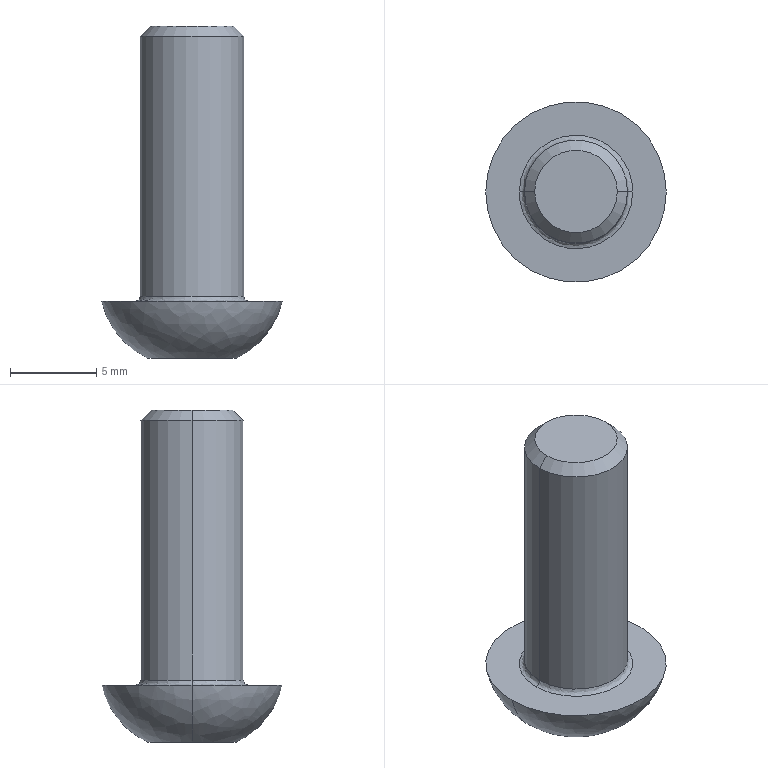Part | SolidWorks | features BaseBody 1 | 1 solid | 25 faces | box 10.5 x 10.5 x 19.3 mm | volume 617.652 mm3 | plane 15 | spline 4 | cone 4 | cylinder 2 | commonest cylinder face diameters 6 x2
STEP:
#1=CARTESIAN_POINT('',(3.,0.,3.6));
#2=VERTEX_POINT('',#1);
#3=CARTESIAN_POINT('',(-3.,0.,3.6));
#4=VERTEX_POINT('',#3);
#5=CARTESIAN_POINT('',(0.,0.,3.6));
#6=DIRECTION('',(0.,0.,1.));
#7=DIRECTION('',(-1.,0.,0.));
#8=AXIS2_PLACEMENT_3D('',#5,#6,#7);
#9=CIRCLE('',#8,3.);
#10=EDGE_CURVE('',#2,#4,#9,.T.);
#11=ORIENTED_EDGE('',*,*,#10,.F.);
#12=CARTESIAN_POINT('',(3.3,0.,3.3));
#13=VERTEX_POINT('',#12);
#14=CARTESIAN_POINT('',(3.3,0.,3.6));
#15=DIRECTION('',(0.,-1.,0.));
#16=DIRECTION('',(1.,0.,0.));
#17=AXIS2_PLACEMENT_3D('',#14,#15,#16);
#18=CIRCLE('',#17,0.3);
#19=EDGE_CURVE('',#2,#13,#18,.T.);
#20=ORIENTED_EDGE('',*,*,#19,.T.);
#21=CARTESIAN_POINT('',(-3.3,0.,3.3));
#22=VERTEX_POINT('',#21);
#23=CARTESIAN_POINT('',(-3.3,0.,3.3));
#24=CARTESIAN_POINT('',(-3.3,0.2099,3.3));
#25=CARTESIAN_POINT('',(-3.271,0.5192,3.3));
#26=CARTESIAN_POINT('',(-3.187,0.8702,3.3));
#27=CARTESIAN_POINT('',(-3.132,1.043,3.3));
#28=CARTESIAN_POINT('',(-3.101,1.129,3.3));
#29=CARTESIAN_POINT('',(-3.087,1.166,3.3));
#30=CARTESIAN_POINT('',(-3.078,1.19,3.3));
#31=CARTESIAN_POINT('',(-3.074,1.201,3.3));
#32=CARTESIAN_POINT('',(-2.9,1.639,3.3));
#33=CARTESIAN_POINT('',(-2.656,2.011,3.3));
#34=CARTESIAN_POINT('',(-2.172,2.495,3.3));
#35=CARTESIAN_POINT('',(-1.911,2.707,3.3));
#36=CARTESIAN_POINT('',(-1.574,2.905,3.3));
#37=CARTESIAN_POINT('',(-1.397,2.991,3.3));
#38=CARTESIAN_POINT('',(-1.32,3.025,3.3));
#39=CARTESIAN_POINT('',(-1.267,3.047,3.3));
#40=CARTESIAN_POINT('',(-1.239,3.059,3.3));
#41=CARTESIAN_POINT('',(-0.8242,3.223,3.3));
#42=CARTESIAN_POINT('',(-0.42,3.3,3.3));
#43=CARTESIAN_POINT('',(0.21,3.3,3.3));
#44=CARTESIAN_POINT('',(0.5193,3.271,3.3));
#45=CARTESIAN_POINT('',(0.8703,3.187,3.3));
#46=CARTESIAN_POINT('',(1.043,3.132,3.3));
#47=CARTESIAN_POINT('',(1.129,3.101,3.3));
#48=CARTESIAN_POINT('',(1.166,3.087,3.3));
#49=CARTESIAN_POINT('',(1.19,3.078,3.3));
#50=CARTESIAN_POINT('',(1.201,3.074,3.3));
#51=CARTESIAN_POINT('',(1.639,2.9,3.3));
#52=CARTESIAN_POINT('',(2.011,2.656,3.3));
#53=CARTESIAN_POINT('',(2.495,2.172,3.3));
#54=CARTESIAN_POINT('',(2.707,1.911,3.3));
#55=CARTESIAN_POINT('',(2.905,1.574,3.3));
#56=CARTESIAN_POINT('',(2.991,1.397,3.3));
#57=CARTESIAN_POINT('',(3.025,1.32,3.3));
#58=CARTESIAN_POINT('',(3.047,1.267,3.3));
#59=CARTESIAN_POINT('',(3.059,1.239,3.3));
#60=CARTESIAN_POINT('',(3.223,0.8244,3.3));
#61=CARTESIAN_POINT('',(3.3,0.4195,3.3));
#62=CARTESIAN_POINT('',(3.3,0.,3.3));
#63=B_SPLINE_CURVE_WITH_KNOTS('',3,(#23,#24,#25,#26,#27,#28,#29,#30,#31,#32,#33,#34,#35,#36,#37,#38,#39,#40,#41,#42,#43,#44,#45,#46,#47,#48,#49,#50,#51,#52,#53,#54,#55,#56,#57,#58,#59,#60,#61,#62),.UNSPECIFIED.,.F.,.F.,(4,1,1,1,1,2,2,2,1,1,1,2,2,2,1,1,1,1,2,2,2,1,1,1,2,2,4),(0.,0.0625,0.09375,0.1094,0.1172,0.1211,0.125,0.25,0.3125,0.3437,0.3594,0.3672,0.375,0.5,0.5625,0.5937,0.6094,0.6172,0.6211,0.625,0.75,0.8125,0.8437,0.8594,0.8672,0.875,1.),.UNSPECIFIED.);
#64=EDGE_CURVE('',#22,#13,#63,.T.);
#65=ORIENTED_EDGE('',*,*,#64,.F.);
#66=CARTESIAN_POINT('',(-3.3,0.,3.6));
#67=DIRECTION('',(0.,1.,0.));
#68=DIRECTION('',(-1.,0.,0.));
#69=AXIS2_PLACEMENT_3D('',#66,#67,#68);
#70=CIRCLE('',#69,0.3);
#71=EDGE_CURVE('',#4,#22,#70,.T.);
#72=ORIENTED_EDGE('',*,*,#71,.F.);
#73=EDGE_LOOP('',(#11,#20,#65,#72));
#74=FACE_OUTER_BOUND('',#73,.T.);
#75=CARTESIAN_POINT('',(-3.,0.,3.6));
#76=CARTESIAN_POINT('',(-3.,6.,3.6));
#77=CARTESIAN_POINT('',(3.,6.,3.6));
#78=CARTESIAN_POINT('',(3.,0.,3.6));
#79=CARTESIAN_POINT('',(-3.,0.,3.424));
#80=CARTESIAN_POINT('',(-3.,6.,3.424));
#81=CARTESIAN_POINT('',(3.,6.,3.424));
#82=CARTESIAN_POINT('',(3.,0.,3.424));
#83=CARTESIAN_POINT('',(-3.124,0.,3.3));
#84=CARTESIAN_POINT('',(-3.124,6.249,3.3));
#85=CARTESIAN_POINT('',(3.124,6.249,3.3));
#86=CARTESIAN_POINT('',(3.124,0.,3.3));
#87=CARTESIAN_POINT('',(-3.3,0.,3.3));
#88=CARTESIAN_POINT('',(-3.3,6.6,3.3));
#89=CARTESIAN_POINT('',(3.3,6.6,3.3));
#90=CARTESIAN_POINT('',(3.3,0.,3.3));
#91=(BOUNDED_SURFACE()B_SPLINE_SURFACE(3,3,((#75,#76,#77,#78),(#79,#80,#81,#82),(#83,#84,#85,#86),(#87,#88,#89,#90)),.UNSPECIFIED.,.F.,.F.,.F.)B_SPLINE_SURFACE_WITH_KNOTS((4,4),(4,4),(0.,1.),(0.,1.),.UNSPECIFIED.)GEOMETRIC_REPRESENTATION_ITEM()RATIONAL_B_SPLINE_SURFACE(((1.,0.3333,0.3333,1.),(0.8047,0.2682,0.2682,0.8047),(0.8047,0.2682,0.2682,0.8047),(1.,0.3333,0.3333,1.)))REPRESENTATION_ITEM('')SURFACE());
#92=ADVANCED_FACE('',(#74),#91,.F.);
#93=CARTESIAN_POINT('',(5.25,0.,3.3));
#94=VERTEX_POINT('',#93);
#95=CARTESIAN_POINT('',(-5.25,0.,3.3));
#96=VERTEX_POINT('',#95);
#97=CARTESIAN_POINT('',(0.,0.,3.3));
#98=DIRECTION('',(0.,0.,-1.));
#99=DIRECTION('',(1.,0.,0.));
#100=AXIS2_PLACEMENT_3D('',#97,#98,#99);
#101=CIRCLE('',#100,5.25);
#102=EDGE_CURVE('',#94,#96,#101,.T.);
#103=ORIENTED_EDGE('',*,*,#102,.T.);
#104=CARTESIAN_POINT('',(-2.6,0.,0.));
#105=VERTEX_POINT('',#104);
#106=CARTESIAN_POINT('',(-0.5657,0.,4.348));
#107=DIRECTION('',(0.,-1.,0.));
#108=DIRECTION('',(-1.,0.,0.));
#109=AXIS2_PLACEMENT_3D('',#106,#107,#108);
#110=CIRCLE('',#109,4.8);
#111=EDGE_CURVE('',#96,#105,#110,.T.);
#112=ORIENTED_EDGE('',*,*,#111,.T.);
#113=CARTESIAN_POINT('',(2.6,0.,0.));
#114=VERTEX_POINT('',#113);
#115=CARTESIAN_POINT('',(0.,0.,0.));
#116=DIRECTION('',(0.,0.,1.));
#117=DIRECTION('',(1.,0.,0.));
#118=AXIS2_PLACEMENT_3D('',#115,#116,#117);
#119=CIRCLE('',#118,2.6);
#120=EDGE_CURVE('',#105,#114,#119,.T.);
#121=ORIENTED_EDGE('',*,*,#120,.T.);
#122=CARTESIAN_POINT('',(0.5657,0.,4.348));
#123=DIRECTION('',(0.,1.,0.));
#124=DIRECTION('',(1.,0.,0.));
#125=AXIS2_PLACEMENT_3D('',#122,#123,#124);
#126=CIRCLE('',#125,4.8);
#127=EDGE_CURVE('',#94,#114,#126,.T.);
#128=ORIENTED_EDGE('',*,*,#127,.F.);
#129=EDGE_LOOP('',(#103,#112,#121,#128));
#130=FACE_OUTER_BOUND('',#129,.T.);
#131=CARTESIAN_POINT('',(-5.25,0.,3.3));
#132=CARTESIAN_POINT('',(-5.25,-10.5,3.3));
#133=CARTESIAN_POINT('',(5.25,-10.5,3.3));
#134=CARTESIAN_POINT('',(5.25,0.,3.3));
#135=CARTESIAN_POINT('',(-4.92,0.,1.822));
#136=CARTESIAN_POINT('',(-4.92,-9.839,1.822));
#137=CARTESIAN_POINT('',(4.92,-9.839,1.822));
#138=CARTESIAN_POINT('',(4.92,0.,1.822));
#139=CARTESIAN_POINT('',(-3.971,0.,0.6417));
#140=CARTESIAN_POINT('',(-3.971,-7.943,0.6417));
#141=CARTESIAN_POINT('',(3.971,-7.943,0.6417));
#142=CARTESIAN_POINT('',(3.971,0.,0.6417));
#143=CARTESIAN_POINT('',(-2.6,0.,0.));
#144=CARTESIAN_POINT('',(-2.6,-5.2,0.));
#145=CARTESIAN_POINT('',(2.6,-5.2,0.));
#146=CARTESIAN_POINT('',(2.6,0.,0.));
#147=(BOUNDED_SURFACE()B_SPLINE_SURFACE(3,3,((#131,#132,#133,#134),(#135,#136,#137,#138),(#139,#140,#141,#142),(#143,#144,#145,#146)),.UNSPECIFIED.,.F.,.F.,.F.)B_SPLINE_SURFACE_WITH_KNOTS((4,4),(4,4),(0.,1.),(0.,1.),.UNSPECIFIED.)GEOMETRIC_REPRESENTATION_ITEM()RATIONAL_B_SPLINE_SURFACE(((1.,0.3333,0.3333,1.),(0.9317,0.3106,0.3106,0.9317),(0.9317,0.3106,0.3106,0.9317),(1.,0.3333,0.3333,1.)))REPRESENTATION_ITEM('')SURFACE());
#148=ADVANCED_FACE('',(#130),#147,.T.);
#149=CARTESIAN_POINT('',(-3.,0.,18.7));
#150=VERTEX_POINT('',#149);
#151=CARTESIAN_POINT('',(3.,0.,18.7));
#152=VERTEX_POINT('',#151);
#153=CARTESIAN_POINT('',(0.,0.,18.7));
#154=DIRECTION('',(0.,0.,-1.));
#155=DIRECTION('',(-1.,0.,0.));
#156=AXIS2_PLACEMENT_3D('',#153,#154,#155);
#157=CIRCLE('',#156,3.);
#158=EDGE_CURVE('',#150,#152,#157,.T.);
#159=ORIENTED_EDGE('',*,*,#158,.T.);
#160=CARTESIAN_POINT('',(3.,0.,19.3));
#161=DIRECTION('',(0.,0.,-1.));
#162=VECTOR('',#161,1000.);
#163=LINE('',#160,#162);
#164=EDGE_CURVE('',#152,#2,#163,.T.);
#165=ORIENTED_EDGE('',*,*,#164,.T.);
#166=ORIENTED_EDGE('',*,*,#10,.T.);
#167=CARTESIAN_POINT('',(-3.,0.,19.3));
#168=DIRECTION('',(0.,0.,-1.));
#169=VECTOR('',#168,1000.);
#170=LINE('',#167,#169);
#171=EDGE_CURVE('',#150,#4,#170,.T.);
#172=ORIENTED_EDGE('',*,*,#171,.F.);
#173=EDGE_LOOP('',(#159,#165,#166,#172));
#174=FACE_OUTER_BOUND('',#173,.T.);
#175=CARTESIAN_POINT('',(0.,0.,19.3));
#176=DIRECTION('',(0.,0.,-1.));
#177=DIRECTION('',(-1.,0.,0.));
#178=AXIS2_PLACEMENT_3D('',#175,#176,#177);
#179=CYLINDRICAL_SURFACE('',#178,3.);
#180=ADVANCED_FACE('',(#174),#179,.T.);
#181=CARTESIAN_POINT('',(-2.4,0.,19.3));
#182=VERTEX_POINT('',#181);
#183=CARTESIAN_POINT('',(2.4,0.,19.3));
#184=VERTEX_POINT('',#183);
#185=CARTESIAN_POINT('',(0.,0.,19.3));
#186=DIRECTION('',(0.,0.,-1.));
#187=DIRECTION('',(-1.,0.,0.));
#188=AXIS2_PLACEMENT_3D('',#185,#186,#187);
#189=CIRCLE('',#188,2.4);
#190=EDGE_CURVE('',#182,#184,#189,.T.);
#191=ORIENTED_EDGE('',*,*,#190,.T.);
#192=CARTESIAN_POINT('',(3.,0.,18.7));
#193=DIRECTION('',(0.7071,0.,-0.7071));
#194=VECTOR('',#193,1000.);
#195=LINE('',#192,#194);
#196=EDGE_CURVE('',#184,#152,#195,.T.);
#197=ORIENTED_EDGE('',*,*,#196,.T.);
#198=ORIENTED_EDGE('',*,*,#158,.F.);
#199=CARTESIAN_POINT('',(-3.,0.,18.7));
#200=DIRECTION('',(-0.7071,0.,-0.7071));
#201=VECTOR('',#200,1000.);
#202=LINE('',#199,#201);
#203=EDGE_CURVE('',#182,#150,#202,.T.);
#204=ORIENTED_EDGE('',*,*,#203,.F.);
#205=EDGE_LOOP('',(#191,#197,#198,#204));
#206=FACE_OUTER_BOUND('',#205,.T.);
#207=CARTESIAN_POINT('',(0.,0.,18.7));
#208=DIRECTION('',(0.,0.,-1.));
#209=DIRECTION('',(-1.,0.,0.));
#210=AXIS2_PLACEMENT_3D('',#207,#208,#209);
#211=CONICAL_SURFACE('',#210,3.,0.7854);
#212=ADVANCED_FACE('',(#206),#211,.T.);
#213=CARTESIAN_POINT('',(0.,0.,3.235));
#214=VERTEX_POINT('',#213);
#215=CARTESIAN_POINT('',(-2.,0.,2.08));
#216=VERTEX_POINT('',#215);
#217=CARTESIAN_POINT('',(-2.,0.,2.08));
#218=DIRECTION('',(-0.866,0.,-0.5));
#219=VECTOR('',#218,1000.);
#220=LINE('',#217,#219);
#221=EDGE_CURVE('',#214,#216,#220,.T.);
#222=ORIENTED_EDGE('',*,*,#221,.F.);
#223=CARTESIAN_POINT('',(2.,0.,2.08));
#224=VERTEX_POINT('',#223);
#225=CARTESIAN_POINT('',(2.,0.,2.08));
#226=DIRECTION('',(0.866,0.,-0.5));
#227=VECTOR('',#226,1000.);
#228=LINE('',#225,#227);
#229=EDGE_CURVE('',#214,#224,#228,.T.);
#230=ORIENTED_EDGE('',*,*,#229,.T.);
#231=CARTESIAN_POINT('',(1.,-1.732,2.08));
#232=VERTEX_POINT('',#231);
#233=CARTESIAN_POINT('',(0.,0.,2.08));
#234=DIRECTION('',(0.,0.,1.));
#235=DIRECTION('',(-1.,0.,0.));
#236=AXIS2_PLACEMENT_3D('',#233,#234,#235);
#237=CIRCLE('',#236,2.);
#238=EDGE_CURVE('',#232,#224,#237,.T.);
#239=ORIENTED_EDGE('',*,*,#238,.F.);
#240=CARTESIAN_POINT('',(-1.,-1.732,2.08));
#241=VERTEX_POINT('',#240);
#242=CARTESIAN_POINT('',(0.,0.,2.08));
#243=DIRECTION('',(0.,0.,1.));
#244=DIRECTION('',(-1.,0.,0.));
#245=AXIS2_PLACEMENT_3D('',#242,#243,#244);
#246=CIRCLE('',#245,2.);
#247=EDGE_CURVE('',#241,#232,#246,.T.);
#248=ORIENTED_EDGE('',*,*,#247,.F.);
#249=CARTESIAN_POINT('',(0.,0.,2.08));
#250=DIRECTION('',(0.,0.,1.));
#251=DIRECTION('',(-1.,0.,0.));
#252=AXIS2_PLACEMENT_3D('',#249,#250,#251);
#253=CIRCLE('',#252,2.);
#254=EDGE_CURVE('',#216,#241,#253,.T.);
#255=ORIENTED_EDGE('',*,*,#254,.F.);
#256=EDGE_LOOP('',(#222,#230,#239,#248,#255));
#257=FACE_OUTER_BOUND('',#256,.T.);
#258=CARTESIAN_POINT('',(0.,0.,2.08));
#259=DIRECTION('',(0.,0.,-1.));
#260=DIRECTION('',(-1.,0.,0.));
#261=AXIS2_PLACEMENT_3D('',#258,#259,#260);
#262=CONICAL_SURFACE('',#261,2.,1.047);
#263=ADVANCED_FACE('',(#257),#262,.F.);
#264=ORIENTED_EDGE('',*,*,#164,.F.);
#265=CARTESIAN_POINT('',(0.,0.,18.7));
#266=DIRECTION('',(0.,0.,-1.));
#267=DIRECTION('',(-1.,0.,0.));
#268=AXIS2_PLACEMENT_3D('',#265,#266,#267);
#269=CIRCLE('',#268,3.);
#270=EDGE_CURVE('',#152,#150,#269,.T.);
#271=ORIENTED_EDGE('',*,*,#270,.T.);
#272=ORIENTED_EDGE('',*,*,#171,.T.);
#273=CARTESIAN_POINT('',(0.,0.,3.6));
#274=DIRECTION('',(0.,0.,1.));
#275=DIRECTION('',(-1.,0.,0.));
#276=AXIS2_PLACEMENT_3D('',#273,#274,#275);
#277=CIRCLE('',#276,3.);
#278=EDGE_CURVE('',#4,#2,#277,.T.);
#279=ORIENTED_EDGE('',*,*,#278,.T.);
#280=EDGE_LOOP('',(#264,#271,#272,#279));
#281=FACE_OUTER_BOUND('',#280,.T.);
#282=CARTESIAN_POINT('',(0.,0.,19.3));
#283=DIRECTION('',(0.,0.,-1.));
#284=DIRECTION('',(-1.,0.,0.));
#285=AXIS2_PLACEMENT_3D('',#282,#283,#284);
#286=CYLINDRICAL_SURFACE('',#285,3.);
#287=ADVANCED_FACE('',(#281),#286,.T.);
#288=ORIENTED_EDGE('',*,*,#19,.F.);
#289=ORIENTED_EDGE('',*,*,#278,.F.);
#290=ORIENTED_EDGE('',*,*,#71,.T.);
#291=CARTESIAN_POINT('',(3.3,0.,3.3));
#292=CARTESIAN_POINT('',(3.3,-0.2099,3.3));
#293=CARTESIAN_POINT('',(3.271,-0.5192,3.3));
#294=CARTESIAN_POINT('',(3.187,-0.8702,3.3));
#295=CARTESIAN_POINT('',(3.132,-1.043,3.3));
#296=CARTESIAN_POINT('',(3.101,-1.129,3.3));
#297=CARTESIAN_POINT('',(3.087,-1.166,3.3));
#298=CARTESIAN_POINT('',(3.078,-1.19,3.3));
#299=CARTESIAN_POINT('',(3.074,-1.201,3.3));
#300=CARTESIAN_POINT('',(2.9,-1.639,3.3));
#301=CARTESIAN_POINT('',(2.656,-2.011,3.3));
#302=CARTESIAN_POINT('',(2.172,-2.495,3.3));
#303=CARTESIAN_POINT('',(1.911,-2.707,3.3));
#304=CARTESIAN_POINT('',(1.574,-2.905,3.3));
#305=CARTESIAN_POINT('',(1.397,-2.991,3.3));
#306=CARTESIAN_POINT('',(1.32,-3.025,3.3));
#307=CARTESIAN_POINT('',(1.267,-3.047,3.3));
#308=CARTESIAN_POINT('',(1.239,-3.059,3.3));
#309=CARTESIAN_POINT('',(0.8242,-3.223,3.3));
#310=CARTESIAN_POINT('',(0.42,-3.3,3.3));
#311=CARTESIAN_POINT('',(-0.21,-3.3,3.3));
#312=CARTESIAN_POINT('',(-0.5193,-3.271,3.3));
#313=CARTESIAN_POINT('',(-0.8703,-3.187,3.3));
#314=CARTESIAN_POINT('',(-1.043,-3.132,3.3));
#315=CARTESIAN_POINT('',(-1.129,-3.101,3.3));
#316=CARTESIAN_POINT('',(-1.166,-3.087,3.3));
#317=CARTESIAN_POINT('',(-1.19,-3.078,3.3));
#318=CARTESIAN_POINT('',(-1.201,-3.074,3.3));
#319=CARTESIAN_POINT('',(-1.639,-2.9,3.3));
#320=CARTESIAN_POINT('',(-2.011,-2.656,3.3));
#321=CARTESIAN_POINT('',(-2.495,-2.172,3.3));
#322=CARTESIAN_POINT('',(-2.707,-1.911,3.3));
#323=CARTESIAN_POINT('',(-2.905,-1.574,3.3));
#324=CARTESIAN_POINT('',(-2.991,-1.397,3.3));
#325=CARTESIAN_POINT('',(-3.025,-1.32,3.3));
#326=CARTESIAN_POINT('',(-3.047,-1.267,3.3));
#327=CARTESIAN_POINT('',(-3.059,-1.239,3.3));
#328=CARTESIAN_POINT('',(-3.223,-0.8244,3.3));
#329=CARTESIAN_POINT('',(-3.3,-0.4195,3.3));
#330=CARTESIAN_POINT('',(-3.3,0.,3.3));
#331=B_SPLINE_CURVE_WITH_KNOTS('',3,(#291,#292,#293,#294,#295,#296,#297,#298,#299,#300,#301,#302,#303,#304,#305,#306,#307,#308,#309,#310,#311,#312,#313,#314,#315,#316,#317,#318,#319,#320,#321,#322,#323,#324,#325,#326,#327,#328,#329,#330),.UNSPECIFIED.,.F.,.F.,(4,1,1,1,1,2,2,2,1,1,1,2,2,2,1,1,1,1,2,2,2,1,1,1,2,2,4),(0.,0.0625,0.09375,0.1094,0.1172,0.1211,0.125,0.25,0.3125,0.3437,0.3594,0.3672,0.375,0.5,0.5625,0.5937,0.6094,0.6172,0.6211,0.625,0.75,0.8125,0.8438,0.8594,0.8672,0.875,1.),.UNSPECIFIED.);
#332=EDGE_CURVE('',#13,#22,#331,.T.);
#333=ORIENTED_EDGE('',*,*,#332,.F.);
#334=EDGE_LOOP('',(#288,#289,#290,#333));
#335=FACE_OUTER_BOUND('',#334,.T.);
#336=CARTESIAN_POINT('',(3.,0.,3.6));
#337=CARTESIAN_POINT('',(3.,-6.,3.6));
#338=CARTESIAN_POINT('',(-3.,-6.,3.6));
#339=CARTESIAN_POINT('',(-3.,0.,3.6));
#340=CARTESIAN_POINT('',(3.,0.,3.424));
#341=CARTESIAN_POINT('',(3.,-6.,3.424));
#342=CARTESIAN_POINT('',(-3.,-6.,3.424));
#343=CARTESIAN_POINT('',(-3.,0.,3.424));
#344=CARTESIAN_POINT('',(3.124,0.,3.3));
#345=CARTESIAN_POINT('',(3.124,-6.249,3.3));
#346=CARTESIAN_POINT('',(-3.124,-6.249,3.3));
#347=CARTESIAN_POINT('',(-3.124,0.,3.3));
#348=CARTESIAN_POINT('',(3.3,0.,3.3));
#349=CARTESIAN_POINT('',(3.3,-6.6,3.3));
#350=CARTESIAN_POINT('',(-3.3,-6.6,3.3));
#351=CARTESIAN_POINT('',(-3.3,0.,3.3));
#352=(BOUNDED_SURFACE()B_SPLINE_SURFACE(3,3,((#336,#337,#338,#339),(#340,#341,#342,#343),(#344,#345,#346,#347),(#348,#349,#350,#351)),.UNSPECIFIED.,.F.,.F.,.F.)B_SPLINE_SURFACE_WITH_KNOTS((4,4),(4,4),(0.,1.),(0.,1.),.UNSPECIFIED.)GEOMETRIC_REPRESENTATION_ITEM()RATIONAL_B_SPLINE_SURFACE(((1.,0.3333,0.3333,1.),(0.8047,0.2682,0.2682,0.8047),(0.8047,0.2682,0.2682,0.8047),(1.,0.3333,0.3333,1.)))REPRESENTATION_ITEM('')SURFACE());
#353=ADVANCED_FACE('',(#335),#352,.F.);
#354=ORIENTED_EDGE('',*,*,#196,.F.);
#355=CARTESIAN_POINT('',(0.,0.,19.3));
#356=DIRECTION('',(0.,0.,-1.));
#357=DIRECTION('',(-1.,0.,0.));
#358=AXIS2_PLACEMENT_3D('',#355,#356,#357);
#359=CIRCLE('',#358,2.4);
#360=EDGE_CURVE('',#184,#182,#359,.T.);
#361=ORIENTED_EDGE('',*,*,#360,.T.);
#362=ORIENTED_EDGE('',*,*,#203,.T.);
#363=ORIENTED_EDGE('',*,*,#270,.F.);
#364=EDGE_LOOP('',(#354,#361,#362,#363));
#365=FACE_OUTER_BOUND('',#364,.T.);
#366=CARTESIAN_POINT('',(0.,0.,18.7));
#367=DIRECTION('',(0.,0.,-1.));
#368=DIRECTION('',(-1.,0.,0.));
#369=AXIS2_PLACEMENT_3D('',#366,#367,#368);
#370=CONICAL_SURFACE('',#369,3.,0.7854);
#371=ADVANCED_FACE('',(#365),#370,.T.);
#372=ORIENTED_EDGE('',*,*,#102,.F.);
#373=CARTESIAN_POINT('',(0.,0.,3.3));
#374=DIRECTION('',(0.,0.,-1.));
#375=DIRECTION('',(1.,0.,0.));
#376=AXIS2_PLACEMENT_3D('',#373,#374,#375);
#377=CIRCLE('',#376,5.25);
#378=EDGE_CURVE('',#96,#94,#377,.T.);
#379=ORIENTED_EDGE('',*,*,#378,.F.);
#380=EDGE_LOOP('',(#372,#379));
#381=FACE_OUTER_BOUND('',#380,.T.);
#382=ORIENTED_EDGE('',*,*,#332,.T.);
#383=ORIENTED_EDGE('',*,*,#64,.T.);
#384=EDGE_LOOP('',(#382,#383));
#385=FACE_BOUND('',#384,.T.);
#386=CARTESIAN_POINT('',(-5.25,0.,3.3));
#387=DIRECTION('',(0.,0.,-1.));
#388=DIRECTION('',(-1.,0.,0.));
#389=AXIS2_PLACEMENT_3D('',#386,#387,#388);
#390=PLANE('',#389);
#391=ADVANCED_FACE('',(#381,#385),#390,.F.);
#392=ORIENTED_EDGE('',*,*,#190,.F.);
#393=ORIENTED_EDGE('',*,*,#360,.F.);
#394=EDGE_LOOP('',(#392,#393));
#395=FACE_OUTER_BOUND('',#394,.T.);
#396=CARTESIAN_POINT('',(0.,0.,19.3));
#397=DIRECTION('',(0.,0.,1.));
#398=DIRECTION('',(1.,0.,0.));
#399=AXIS2_PLACEMENT_3D('',#396,#397,#398);
#400=PLANE('',#399);
#401=ADVANCED_FACE('',(#395),#400,.T.);
#402=ORIENTED_EDGE('',*,*,#111,.F.);
#403=ORIENTED_EDGE('',*,*,#378,.T.);
#404=ORIENTED_EDGE('',*,*,#127,.T.);
#405=CARTESIAN_POINT('',(0.,0.,0.));
#406=DIRECTION('',(0.,0.,1.));
#407=DIRECTION('',(1.,0.,0.));
#408=AXIS2_PLACEMENT_3D('',#405,#406,#407);
#409=CIRCLE('',#408,2.6);
#410=EDGE_CURVE('',#114,#105,#409,.T.);
#411=ORIENTED_EDGE('',*,*,#410,.T.);
#412=EDGE_LOOP('',(#402,#403,#404,#411));
#413=FACE_OUTER_BOUND('',#412,.T.);
#414=CARTESIAN_POINT('',(5.25,0.,3.3));
#415=CARTESIAN_POINT('',(5.25,10.5,3.3));
#416=CARTESIAN_POINT('',(-5.25,10.5,3.3));
#417=CARTESIAN_POINT('',(-5.25,0.,3.3));
#418=CARTESIAN_POINT('',(4.92,0.,1.822));
#419=CARTESIAN_POINT('',(4.92,9.839,1.822));
#420=CARTESIAN_POINT('',(-4.92,9.839,1.822));
#421=CARTESIAN_POINT('',(-4.92,0.,1.822));
#422=CARTESIAN_POINT('',(3.971,0.,0.6417));
#423=CARTESIAN_POINT('',(3.971,7.943,0.6417));
#424=CARTESIAN_POINT('',(-3.971,7.943,0.6417));
#425=CARTESIAN_POINT('',(-3.971,0.,0.6417));
#426=CARTESIAN_POINT('',(2.6,0.,0.));
#427=CARTESIAN_POINT('',(2.6,5.2,0.));
#428=CARTESIAN_POINT('',(-2.6,5.2,0.));
#429=CARTESIAN_POINT('',(-2.6,0.,0.));
#430=(BOUNDED_SURFACE()B_SPLINE_SURFACE(3,3,((#414,#415,#416,#417),(#418,#419,#420,#421),(#422,#423,#424,#425),(#426,#427,#428,#429)),.UNSPECIFIED.,.F.,.F.,.F.)B_SPLINE_SURFACE_WITH_KNOTS((4,4),(4,4),(0.,1.),(0.,1.),.UNSPECIFIED.)GEOMETRIC_REPRESENTATION_ITEM()RATIONAL_B_SPLINE_SURFACE(((1.,0.3333,0.3333,1.),(0.9317,0.3106,0.3106,0.9317),(0.9317,0.3106,0.3106,0.9317),(1.,0.3333,0.3333,1.)))REPRESENTATION_ITEM('')SURFACE());
#431=ADVANCED_FACE('',(#413),#430,.T.);
#432=ORIENTED_EDGE('',*,*,#410,.F.);
#433=ORIENTED_EDGE('',*,*,#120,.F.);
#434=EDGE_LOOP('',(#432,#433));
#435=FACE_OUTER_BOUND('',#434,.T.);
#436=CARTESIAN_POINT('',(-2.,-1.155,0.));
#437=VERTEX_POINT('',#436);
#438=CARTESIAN_POINT('',(-2.,1.155,0.));
#439=VERTEX_POINT('',#438);
#440=CARTESIAN_POINT('',(-2.,0.,0.));
#441=DIRECTION('',(0.,1.,0.));
#442=VECTOR('',#441,1000.);
#443=LINE('',#440,#442);
#444=EDGE_CURVE('',#437,#439,#443,.T.);
#445=ORIENTED_EDGE('',*,*,#444,.F.);
#446=CARTESIAN_POINT('',(0.,-2.309,0.));
#447=VERTEX_POINT('',#446);
#448=CARTESIAN_POINT('',(0.,-2.309,0.));
#449=DIRECTION('',(-0.866,0.5,0.));
#450=VECTOR('',#449,1000.);
#451=LINE('',#448,#450);
#452=EDGE_CURVE('',#447,#437,#451,.T.);
#453=ORIENTED_EDGE('',*,*,#452,.F.);
#454=CARTESIAN_POINT('',(2.,-1.155,0.));
#455=VERTEX_POINT('',#454);
#456=CARTESIAN_POINT('',(2.,-1.155,0.));
#457=DIRECTION('',(-0.866,-0.5,0.));
#458=VECTOR('',#457,1000.);
#459=LINE('',#456,#458);
#460=EDGE_CURVE('',#455,#447,#459,.T.);
#461=ORIENTED_EDGE('',*,*,#460,.F.);
#462=CARTESIAN_POINT('',(2.,1.155,0.));
#463=VERTEX_POINT('',#462);
#464=CARTESIAN_POINT('',(2.,0.,0.));
#465=DIRECTION('',(0.,-1.,0.));
#466=VECTOR('',#465,1000.);
#467=LINE('',#464,#466);
#468=EDGE_CURVE('',#463,#455,#467,.T.);
#469=ORIENTED_EDGE('',*,*,#468,.F.);
#470=CARTESIAN_POINT('',(0.,2.309,0.));
#471=VERTEX_POINT('',#470);
#472=CARTESIAN_POINT('',(0.,2.309,0.));
#473=DIRECTION('',(0.866,-0.5,0.));
#474=VECTOR('',#473,1000.);
#475=LINE('',#472,#474);
#476=EDGE_CURVE('',#471,#463,#475,.T.);
#477=ORIENTED_EDGE('',*,*,#476,.F.);
#478=CARTESIAN_POINT('',(-2.,1.155,0.));
#479=DIRECTION('',(0.866,0.5,0.));
#480=VECTOR('',#479,1000.);
#481=LINE('',#478,#480);
#482=EDGE_CURVE('',#439,#471,#481,.T.);
#483=ORIENTED_EDGE('',*,*,#482,.F.);
#484=EDGE_LOOP('',(#445,#453,#461,#469,#477,#483));
#485=FACE_BOUND('',#484,.T.);
#486=CARTESIAN_POINT('',(-2.6,0.,0.));
#487=DIRECTION('',(0.,0.,1.));
#488=DIRECTION('',(1.,0.,0.));
#489=AXIS2_PLACEMENT_3D('',#486,#487,#488);
#490=PLANE('',#489);
#491=ADVANCED_FACE('',(#435,#485),#490,.F.);
#492=CARTESIAN_POINT('',(0.,2.309,2.08));
#493=VERTEX_POINT('',#492);
#494=CARTESIAN_POINT('',(0.,2.309,2.08));
#495=DIRECTION('',(0.,0.,-1.));
#496=VECTOR('',#495,1000.);
#497=LINE('',#494,#496);
#498=EDGE_CURVE('',#493,#471,#497,.T.);
#499=ORIENTED_EDGE('',*,*,#498,.F.);
#500=CARTESIAN_POINT('',(-1.,1.732,2.08));
#501=VERTEX_POINT('',#500);
#502=CARTESIAN_POINT('',(-1.,1.732,2.08));
#503=DIRECTION('',(0.866,0.5,0.));
#504=VECTOR('',#503,1000.);
#505=LINE('',#502,#504);
#506=EDGE_CURVE('',#501,#493,#505,.T.);
#507=ORIENTED_EDGE('',*,*,#506,.F.);
#508=CARTESIAN_POINT('',(-2.,1.155,2.08));
#509=VERTEX_POINT('',#508);
#510=CARTESIAN_POINT('',(-2.,1.155,2.08));
#511=DIRECTION('',(0.866,0.5,0.));
#512=VECTOR('',#511,1000.);
#513=LINE('',#510,#512);
#514=EDGE_CURVE('',#509,#501,#513,.T.);
#515=ORIENTED_EDGE('',*,*,#514,.F.);
#516=CARTESIAN_POINT('',(-2.,1.155,2.08));
#517=DIRECTION('',(0.,0.,1.));
#518=VECTOR('',#517,1000.);
#519=LINE('',#516,#518);
#520=EDGE_CURVE('',#439,#509,#519,.T.);
#521=ORIENTED_EDGE('',*,*,#520,.F.);
#522=ORIENTED_EDGE('',*,*,#482,.T.);
#523=EDGE_LOOP('',(#499,#507,#515,#521,#522));
#524=FACE_OUTER_BOUND('',#523,.T.);
#525=CARTESIAN_POINT('',(-2.,1.155,2.08));
#526=DIRECTION('',(-0.5,0.866,0.));
#527=DIRECTION('',(-0.866,-0.5,0.));
#528=AXIS2_PLACEMENT_3D('',#525,#526,#527);
#529=PLANE('',#528);
#530=ADVANCED_FACE('',(#524),#529,.F.);
#531=ORIENTED_EDGE('',*,*,#520,.T.);
#532=CARTESIAN_POINT('',(-2.,0.,2.08));
#533=DIRECTION('',(0.,1.,0.));
#534=VECTOR('',#533,1000.);
#535=LINE('',#532,#534);
#536=EDGE_CURVE('',#216,#509,#535,.T.);
#537=ORIENTED_EDGE('',*,*,#536,.F.);
#538=CARTESIAN_POINT('',(-2.,-1.155,2.08));
#539=VERTEX_POINT('',#538);
#540=CARTESIAN_POINT('',(-2.,0.,2.08));
#541=DIRECTION('',(0.,1.,0.));
#542=VECTOR('',#541,1000.);
#543=LINE('',#540,#542);
#544=EDGE_CURVE('',#539,#216,#543,.T.);
#545=ORIENTED_EDGE('',*,*,#544,.F.);
#546=CARTESIAN_POINT('',(-2.,-1.155,2.08));
#547=DIRECTION('',(0.,0.,1.));
#548=VECTOR('',#547,1000.);
#549=LINE('',#546,#548);
#550=EDGE_CURVE('',#437,#539,#549,.T.);
#551=ORIENTED_EDGE('',*,*,#550,.F.);
#552=ORIENTED_EDGE('',*,*,#444,.T.);
#553=EDGE_LOOP('',(#531,#537,#545,#551,#552));
#554=FACE_OUTER_BOUND('',#553,.T.);
#555=CARTESIAN_POINT('',(-2.,-1.155,2.08));
#556=DIRECTION('',(-1.,0.,0.));
#557=DIRECTION('',(0.,0.,1.));
#558=AXIS2_PLACEMENT_3D('',#555,#556,#557);
#559=PLANE('',#558);
#560=ADVANCED_FACE('',(#554),#559,.F.);
#561=ORIENTED_EDGE('',*,*,#550,.T.);
#562=CARTESIAN_POINT('',(-1.,-1.732,2.08));
#563=DIRECTION('',(-0.866,0.5,0.));
#564=VECTOR('',#563,1000.);
#565=LINE('',#562,#564);
#566=EDGE_CURVE('',#241,#539,#565,.T.);
#567=ORIENTED_EDGE('',*,*,#566,.F.);
#568=CARTESIAN_POINT('',(0.,-2.309,2.08));
#569=VERTEX_POINT('',#568);
#570=CARTESIAN_POINT('',(0.,-2.309,2.08));
#571=DIRECTION('',(-0.866,0.5,0.));
#572=VECTOR('',#571,1000.);
#573=LINE('',#570,#572);
#574=EDGE_CURVE('',#569,#241,#573,.T.);
#575=ORIENTED_EDGE('',*,*,#574,.F.);
#576=CARTESIAN_POINT('',(0.,-2.309,2.08));
#577=DIRECTION('',(0.,0.,1.));
#578=VECTOR('',#577,1000.);
#579=LINE('',#576,#578);
#580=EDGE_CURVE('',#447,#569,#579,.T.);
#581=ORIENTED_EDGE('',*,*,#580,.F.);
#582=ORIENTED_EDGE('',*,*,#452,.T.);
#583=EDGE_LOOP('',(#561,#567,#575,#581,#582));
#584=FACE_OUTER_BOUND('',#583,.T.);
#585=CARTESIAN_POINT('',(0.,-2.309,2.08));
#586=DIRECTION('',(-0.5,-0.866,0.));
#587=DIRECTION('',(0.866,-0.5,0.));
#588=AXIS2_PLACEMENT_3D('',#585,#586,#587);
#589=PLANE('',#588);
#590=ADVANCED_FACE('',(#584),#589,.F.);
#591=ORIENTED_EDGE('',*,*,#580,.T.);
#592=CARTESIAN_POINT('',(1.,-1.732,2.08));
#593=DIRECTION('',(-0.866,-0.5,0.));
#594=VECTOR('',#593,1000.);
#595=LINE('',#592,#594);
#596=EDGE_CURVE('',#232,#569,#595,.T.);
#597=ORIENTED_EDGE('',*,*,#596,.F.);
#598=CARTESIAN_POINT('',(2.,-1.155,2.08));
#599=VERTEX_POINT('',#598);
#600=CARTESIAN_POINT('',(2.,-1.155,2.08));
#601=DIRECTION('',(-0.866,-0.5,0.));
#602=VECTOR('',#601,1000.);
#603=LINE('',#600,#602);
#604=EDGE_CURVE('',#599,#232,#603,.T.);
#605=ORIENTED_EDGE('',*,*,#604,.F.);
#606=CARTESIAN_POINT('',(2.,-1.155,2.08));
#607=DIRECTION('',(0.,0.,1.));
#608=VECTOR('',#607,1000.);
#609=LINE('',#606,#608);
#610=EDGE_CURVE('',#455,#599,#609,.T.);
#611=ORIENTED_EDGE('',*,*,#610,.F.);
#612=ORIENTED_EDGE('',*,*,#460,.T.);
#613=EDGE_LOOP('',(#591,#597,#605,#611,#612));
#614=FACE_OUTER_BOUND('',#613,.T.);
#615=CARTESIAN_POINT('',(2.,-1.155,2.08));
#616=DIRECTION('',(0.5,-0.866,0.));
#617=DIRECTION('',(0.866,0.5,0.));
#618=AXIS2_PLACEMENT_3D('',#615,#616,#617);
#619=PLANE('',#618);
#620=ADVANCED_FACE('',(#614),#619,.F.);
#621=ORIENTED_EDGE('',*,*,#610,.T.);
#622=CARTESIAN_POINT('',(2.,0.,2.08));
#623=DIRECTION('',(0.,-1.,0.));
#624=VECTOR('',#623,1000.);
#625=LINE('',#622,#624);
#626=EDGE_CURVE('',#224,#599,#625,.T.);
#627=ORIENTED_EDGE('',*,*,#626,.F.);
#628=CARTESIAN_POINT('',(2.,1.155,2.08));
#629=VERTEX_POINT('',#628);
#630=CARTESIAN_POINT('',(2.,0.,2.08));
#631=DIRECTION('',(0.,-1.,0.));
#632=VECTOR('',#631,1000.);
#633=LINE('',#630,#632);
#634=EDGE_CURVE('',#629,#224,#633,.T.);
#635=ORIENTED_EDGE('',*,*,#634,.F.);
#636=CARTESIAN_POINT('',(2.,1.155,2.08));
#637=DIRECTION('',(0.,0.,1.));
#638=VECTOR('',#637,1000.);
#639=LINE('',#636,#638);
#640=EDGE_CURVE('',#463,#629,#639,.T.);
#641=ORIENTED_EDGE('',*,*,#640,.F.);
#642=ORIENTED_EDGE('',*,*,#468,.T.);
#643=EDGE_LOOP('',(#621,#627,#635,#641,#642));
#644=FACE_OUTER_BOUND('',#643,.T.);
#645=CARTESIAN_POINT('',(2.,1.155,2.08));
#646=DIRECTION('',(1.,0.,0.));
#647=DIRECTION('',(0.,0.,-1.));
#648=AXIS2_PLACEMENT_3D('',#645,#646,#647);
#649=PLANE('',#648);
#650=ADVANCED_FACE('',(#644),#649,.F.);
#651=ORIENTED_EDGE('',*,*,#640,.T.);
#652=CARTESIAN_POINT('',(1.,1.732,2.08));
#653=VERTEX_POINT('',#652);
#654=CARTESIAN_POINT('',(0.,2.309,2.08));
#655=DIRECTION('',(0.866,-0.5,0.));
#656=VECTOR('',#655,1000.);
#657=LINE('',#654,#656);
#658=EDGE_CURVE('',#653,#629,#657,.T.);
#659=ORIENTED_EDGE('',*,*,#658,.F.);
#660=CARTESIAN_POINT('',(0.,2.309,2.08));
#661=DIRECTION('',(0.866,-0.5,0.));
#662=VECTOR('',#661,1000.);
#663=LINE('',#660,#662);
#664=EDGE_CURVE('',#493,#653,#663,.T.);
#665=ORIENTED_EDGE('',*,*,#664,.F.);
#666=ORIENTED_EDGE('',*,*,#498,.T.);
#667=ORIENTED_EDGE('',*,*,#476,.T.);
#668=EDGE_LOOP('',(#651,#659,#665,#666,#667));
#669=FACE_OUTER_BOUND('',#668,.T.);
#670=CARTESIAN_POINT('',(0.,2.309,2.08));
#671=DIRECTION('',(0.5,0.866,0.));
#672=DIRECTION('',(-0.866,0.5,0.));
#673=AXIS2_PLACEMENT_3D('',#670,#671,#672);
#674=PLANE('',#673);
#675=ADVANCED_FACE('',(#669),#674,.F.);
#676=ORIENTED_EDGE('',*,*,#658,.T.);
#677=ORIENTED_EDGE('',*,*,#634,.T.);
#678=CARTESIAN_POINT('',(0.,0.,2.08));
#679=DIRECTION('',(0.,0.,1.));
#680=DIRECTION('',(-1.,0.,0.));
#681=AXIS2_PLACEMENT_3D('',#678,#679,#680);
#682=CIRCLE('',#681,2.);
#683=EDGE_CURVE('',#224,#653,#682,.T.);
#684=ORIENTED_EDGE('',*,*,#683,.T.);
#685=EDGE_LOOP('',(#676,#677,#684));
#686=FACE_OUTER_BOUND('',#685,.T.);
#687=CARTESIAN_POINT('',(0.,0.,2.08));
#688=DIRECTION('',(0.,0.,-1.));
#689=DIRECTION('',(-1.,0.,0.));
#690=AXIS2_PLACEMENT_3D('',#687,#688,#689);
#691=PLANE('',#690);
#692=ADVANCED_FACE('',(#686),#691,.T.);
#693=ORIENTED_EDGE('',*,*,#229,.F.);
#694=ORIENTED_EDGE('',*,*,#221,.T.);
#695=CARTESIAN_POINT('',(0.,0.,2.08));
#696=DIRECTION('',(0.,0.,1.));
#697=DIRECTION('',(-1.,0.,0.));
#698=AXIS2_PLACEMENT_3D('',#695,#696,#697);
#699=CIRCLE('',#698,2.);
#700=EDGE_CURVE('',#501,#216,#699,.T.);
#701=ORIENTED_EDGE('',*,*,#700,.F.);
#702=CARTESIAN_POINT('',(0.,0.,2.08));
#703=DIRECTION('',(0.,0.,1.));
#704=DIRECTION('',(-1.,0.,0.));
#705=AXIS2_PLACEMENT_3D('',#702,#703,#704);
#706=CIRCLE('',#705,2.);
#707=EDGE_CURVE('',#653,#501,#706,.T.);
#708=ORIENTED_EDGE('',*,*,#707,.F.);
#709=ORIENTED_EDGE('',*,*,#683,.F.);
#710=EDGE_LOOP('',(#693,#694,#701,#708,#709));
#711=FACE_OUTER_BOUND('',#710,.T.);
#712=CARTESIAN_POINT('',(0.,0.,2.08));
#713=DIRECTION('',(0.,0.,-1.));
#714=DIRECTION('',(-1.,0.,0.));
#715=AXIS2_PLACEMENT_3D('',#712,#713,#714);
#716=CONICAL_SURFACE('',#715,2.,1.047);
#717=ADVANCED_FACE('',(#711),#716,.F.);
#718=ORIENTED_EDGE('',*,*,#536,.T.);
#719=ORIENTED_EDGE('',*,*,#514,.T.);
#720=ORIENTED_EDGE('',*,*,#700,.T.);
#721=EDGE_LOOP('',(#718,#719,#720));
#722=FACE_OUTER_BOUND('',#721,.T.);
#723=CARTESIAN_POINT('',(0.,0.,2.08));
#724=DIRECTION('',(0.,0.,-1.));
#725=DIRECTION('',(-1.,0.,0.));
#726=AXIS2_PLACEMENT_3D('',#723,#724,#725);
#727=PLANE('',#726);
#728=ADVANCED_FACE('',(#722),#727,.T.);
#729=ORIENTED_EDGE('',*,*,#506,.T.);
#730=ORIENTED_EDGE('',*,*,#664,.T.);
#731=ORIENTED_EDGE('',*,*,#707,.T.);
#732=EDGE_LOOP('',(#729,#730,#731));
#733=FACE_OUTER_BOUND('',#732,.T.);
#734=CARTESIAN_POINT('',(0.,0.,2.08));
#735=DIRECTION('',(0.,0.,-1.));
#736=DIRECTION('',(-1.,0.,0.));
#737=AXIS2_PLACEMENT_3D('',#734,#735,#736);
#738=PLANE('',#737);
#739=ADVANCED_FACE('',(#733),#738,.T.);
#740=ORIENTED_EDGE('',*,*,#626,.T.);
#741=ORIENTED_EDGE('',*,*,#604,.T.);
#742=ORIENTED_EDGE('',*,*,#238,.T.);
#743=EDGE_LOOP('',(#740,#741,#742));
#744=FACE_OUTER_BOUND('',#743,.T.);
#745=CARTESIAN_POINT('',(0.,0.,2.08));
#746=DIRECTION('',(0.,0.,-1.));
#747=DIRECTION('',(-1.,0.,0.));
#748=AXIS2_PLACEMENT_3D('',#745,#746,#747);
#749=PLANE('',#748);
#750=ADVANCED_FACE('',(#744),#749,.T.);
#751=ORIENTED_EDGE('',*,*,#596,.T.);
#752=ORIENTED_EDGE('',*,*,#574,.T.);
#753=ORIENTED_EDGE('',*,*,#247,.T.);
#754=EDGE_LOOP('',(#751,#752,#753));
#755=FACE_OUTER_BOUND('',#754,.T.);
#756=CARTESIAN_POINT('',(0.,0.,2.08));
#757=DIRECTION('',(0.,0.,-1.));
#758=DIRECTION('',(-1.,0.,0.));
#759=AXIS2_PLACEMENT_3D('',#756,#757,#758);
#760=PLANE('',#759);
#761=ADVANCED_FACE('',(#755),#760,.T.);
#762=ORIENTED_EDGE('',*,*,#566,.T.);
#763=ORIENTED_EDGE('',*,*,#544,.T.);
#764=ORIENTED_EDGE('',*,*,#254,.T.);
#765=EDGE_LOOP('',(#762,#763,#764));
#766=FACE_OUTER_BOUND('',#765,.T.);
#767=CARTESIAN_POINT('',(0.,0.,2.08));
#768=DIRECTION('',(0.,0.,-1.));
#769=DIRECTION('',(-1.,0.,0.));
#770=AXIS2_PLACEMENT_3D('',#767,#768,#769);
#771=PLANE('',#770);
#772=ADVANCED_FACE('',(#766),#771,.T.);
#773=CLOSED_SHELL('',(#92,#148,#180,#212,#263,#287,#353,#371,#391,#401,#431,#491,#530,#560,#590,#620,#650,#675,#692,#717,#728,#739,#750,#761,#772));
#774=MANIFOLD_SOLID_BREP('',#773);
#775=CARTESIAN_POINT('',(0.,0.,0.));
#776=DIRECTION('',(0.,0.,1.));
#777=DIRECTION('',(1.,0.,0.));
#778=AXIS2_PLACEMENT_3D('',#775,#776,#777);
#779=(LENGTH_UNIT()NAMED_UNIT(*)SI_UNIT(.MILLI.,.METRE.));
#780=UNCERTAINTY_MEASURE_WITH_UNIT(LENGTH_MEASURE(0.00001),#779,'','');
#781=(NAMED_UNIT(*)PLANE_ANGLE_UNIT()SI_UNIT($,.RADIAN.));
#782=(NAMED_UNIT(*)SI_UNIT($,.STERADIAN.)SOLID_ANGLE_UNIT());
#783=(GEOMETRIC_REPRESENTATION_CONTEXT(3)GLOBAL_UNCERTAINTY_ASSIGNED_CONTEXT((#780))GLOBAL_UNIT_ASSIGNED_CONTEXT((#779,#781,#782))REPRESENTATION_CONTEXT('',''));
#784=ADVANCED_BREP_SHAPE_REPRESENTATION('',(#774,#778),#783);